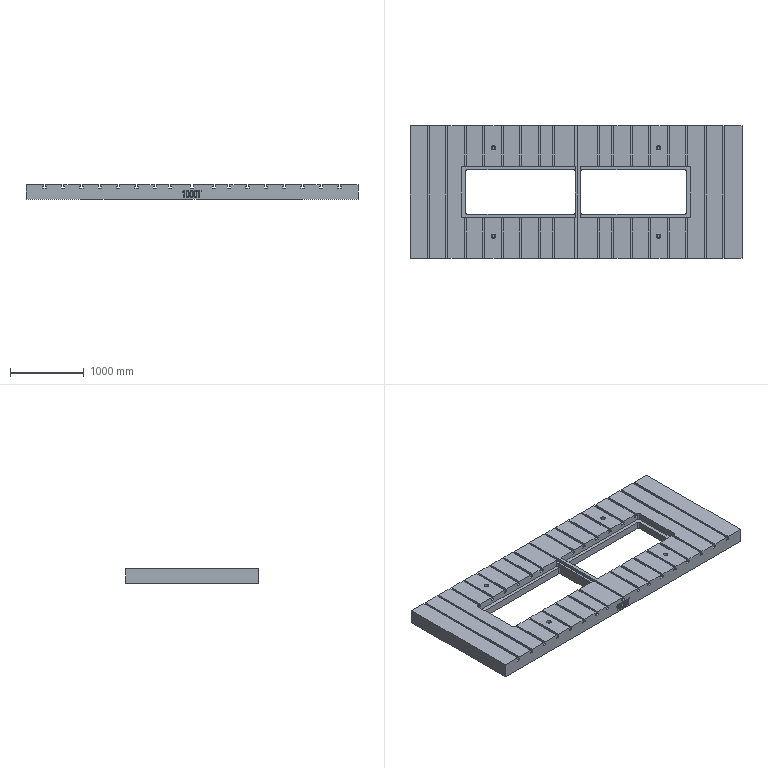Part | STEP file | lll_id5078_x_t | 1 solid | 323 faces | box 4500 x 1800 x 200 mm | volume 1192817738 mm3 | plane 285 | cylinder 24 | other 14 | commonest cylinder face diameters 40 x20 60 x4